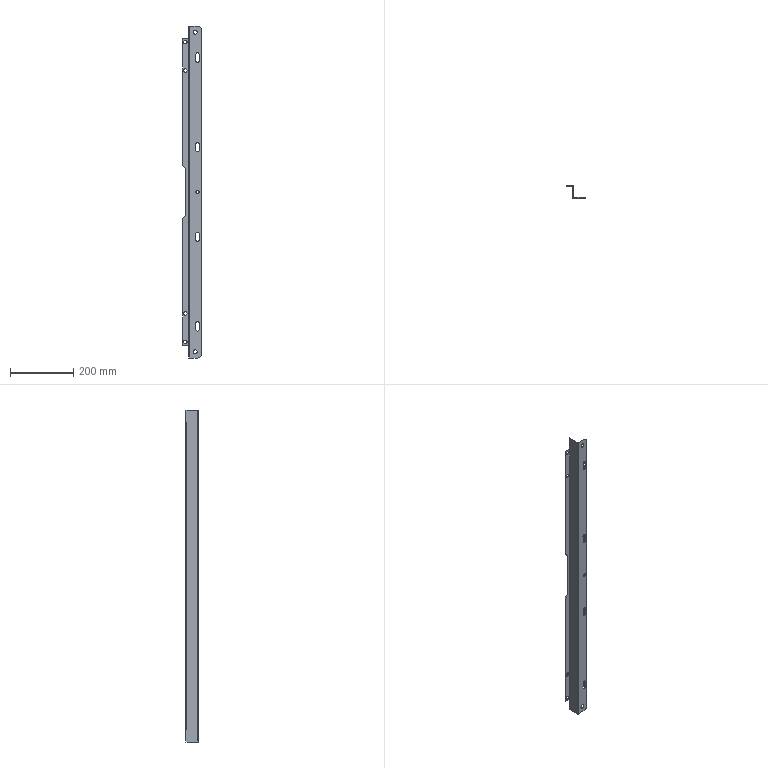Part | SolidWorks | features ICE 3, Cut 2, SMBaseFlange 2, Chamfer 1, Fillet 1, FlatPattern 1, SheetMetal 1 | 1 solid | 70 faces | box 60 x 38 x 1050 mm | volume 143033 mm3 | plane 38 | cylinder 32 | commonest cylinder face diameters 10 x14 11 x8 12.8 x4 0.4 x2 3.4 x2 26 x2